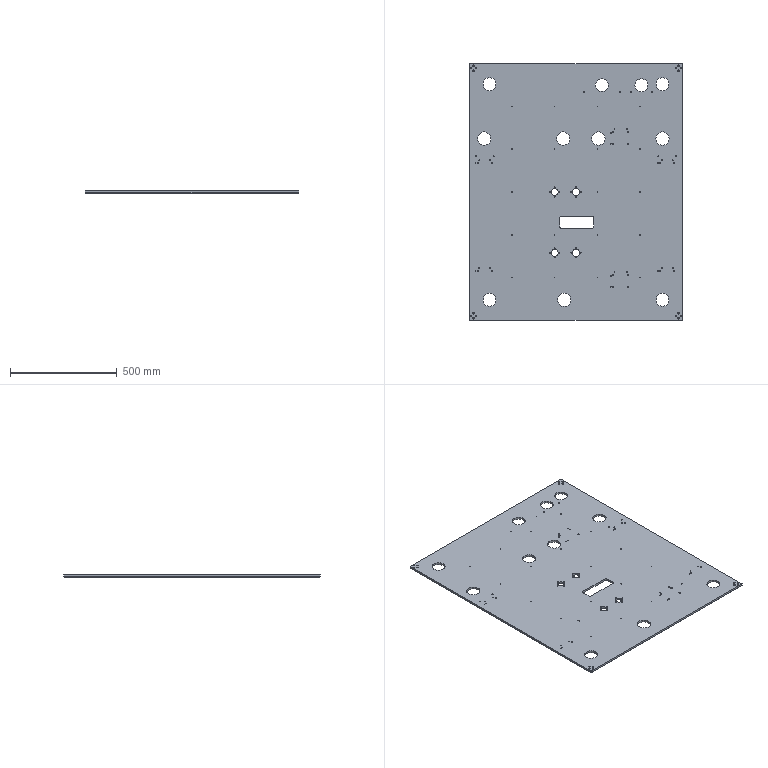Part | STEP file | table plate | 1 solid | 336 faces | box 1000 x 1200 x 10 mm | volume 11534031 mm3 | cylinder 272 | cone 50 | plane 14 | commonest cylinder face diameters 4.2 x80 6.8 x48 6 x40 3.3 x38 5 x24 60.5 x12